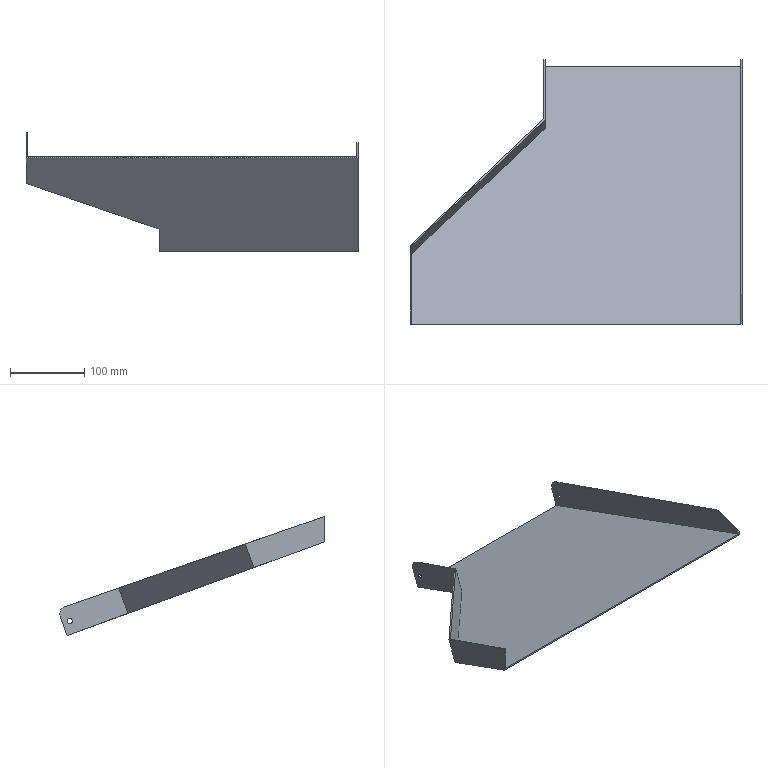Part | NX | features HB 2 | 1 solid | 19 faces | box 446 x 355.386 x 159.875 mm | volume 316995 mm3 | plane 15 | cylinder 4 | commonest cylinder face diameters 7 x2 20 x2
STEP:
#1=CARTESIAN_POINT('',(560.,345.,-264.005));
#2=VERTEX_POINT('',#1);
#3=CARTESIAN_POINT('',(118.,345.,-264.005));
#4=VERTEX_POINT('',#3);
#5=CARTESIAN_POINT('',(650.,345.,-264.005));
#6=DIRECTION('',(-1.,0.,0.));
#7=VECTOR('',#6,1000.);
#8=LINE('',#5,#7);
#9=EDGE_CURVE('',#2,#4,#8,.T.);
#10=ORIENTED_EDGE('',*,*,#9,.F.);
#11=CARTESIAN_POINT('',(560.,691.161,-389.998));
#12=VERTEX_POINT('',#11);
#13=CARTESIAN_POINT('',(560.,379.611,-276.603));
#14=DIRECTION('',(0.,0.9397,-0.342));
#15=VECTOR('',#14,1000.);
#16=LINE('',#13,#15);
#17=EDGE_CURVE('',#2,#12,#16,.T.);
#18=ORIENTED_EDGE('',*,*,#17,.T.);
#19=CARTESIAN_POINT('',(298.,691.161,-389.998));
#20=VERTEX_POINT('',#19);
#21=CARTESIAN_POINT('',(258.,691.161,-389.998));
#22=DIRECTION('',(1.,0.,0.));
#23=VECTOR('',#22,1000.);
#24=LINE('',#21,#23);
#25=EDGE_CURVE('',#20,#12,#24,.T.);
#26=ORIENTED_EDGE('',*,*,#25,.F.);
#27=CARTESIAN_POINT('',(298.,608.554,-359.931));
#28=VERTEX_POINT('',#27);
#29=CARTESIAN_POINT('',(298.,379.611,-276.603));
#30=DIRECTION('',(0.,-0.9397,0.342));
#31=VECTOR('',#30,1000.);
#32=LINE('',#29,#31);
#33=EDGE_CURVE('',#20,#28,#32,.T.);
#34=ORIENTED_EDGE('',*,*,#33,.T.);
#35=CARTESIAN_POINT('',(118.,439.409,-298.367));
#36=VERTEX_POINT('',#35);
#37=CARTESIAN_POINT('',(133.682,454.145,-303.731));
#38=DIRECTION('',(-0.7071,-0.6645,0.2418));
#39=VECTOR('',#38,1000.);
#40=LINE('',#37,#39);
#41=EDGE_CURVE('',#28,#36,#40,.T.);
#42=ORIENTED_EDGE('',*,*,#41,.T.);
#43=CARTESIAN_POINT('',(118.,379.611,-276.603));
#44=DIRECTION('',(0.,-0.9397,0.342));
#45=VECTOR('',#44,1000.);
#46=LINE('',#43,#45);
#47=EDGE_CURVE('',#36,#4,#46,.T.);
#48=ORIENTED_EDGE('',*,*,#47,.T.);
#49=EDGE_LOOP('',(#10,#18,#26,#34,#42,#48));
#50=FACE_BOUND('',#49,.T.);
#51=CARTESIAN_POINT('',(258.,379.611,-276.603));
#52=DIRECTION('',(0.,0.342,0.9397));
#53=DIRECTION('',(1.,0.,0.));
#54=AXIS2_PLACEMENT_3D('',#51,#52,#53);
#55=PLANE('',#54);
#56=ADVANCED_FACE('',(#50),#55,.T.);
#57=CARTESIAN_POINT('',(560.,345.,-260.721));
#58=VERTEX_POINT('',#57);
#59=CARTESIAN_POINT('',(560.,345.,60.));
#60=DIRECTION('',(0.,0.,-1.));
#61=VECTOR('',#60,1000.);
#62=LINE('',#59,#61);
#63=EDGE_CURVE('',#58,#2,#62,.T.);
#64=ORIENTED_EDGE('',*,*,#63,.T.);
#65=ORIENTED_EDGE('',*,*,#9,.T.);
#66=CARTESIAN_POINT('',(118.,345.,-232.002));
#67=VERTEX_POINT('',#66);
#68=CARTESIAN_POINT('',(118.,345.,60.));
#69=DIRECTION('',(0.,0.,1.));
#70=VECTOR('',#69,1000.);
#71=LINE('',#68,#70);
#72=EDGE_CURVE('',#4,#67,#71,.T.);
#73=ORIENTED_EDGE('',*,*,#72,.T.);
#74=CARTESIAN_POINT('',(116.,345.,-232.002));
#75=VERTEX_POINT('',#74);
#76=CARTESIAN_POINT('',(650.,345.,-232.002));
#77=DIRECTION('',(1.,0.,0.));
#78=VECTOR('',#77,1000.);
#79=LINE('',#76,#78);
#80=EDGE_CURVE('',#75,#67,#79,.T.);
#81=ORIENTED_EDGE('',*,*,#80,.F.);
#82=CARTESIAN_POINT('',(116.,345.,-266.134));
#83=VERTEX_POINT('',#82);
#84=CARTESIAN_POINT('',(116.,345.,60.));
#85=DIRECTION('',(0.,0.,1.));
#86=VECTOR('',#85,1000.);
#87=LINE('',#84,#86);
#88=EDGE_CURVE('',#83,#75,#87,.T.);
#89=ORIENTED_EDGE('',*,*,#88,.F.);
#90=CARTESIAN_POINT('',(562.,345.,-266.134));
#91=VERTEX_POINT('',#90);
#92=CARTESIAN_POINT('',(650.,345.,-266.134));
#93=DIRECTION('',(-1.,0.,0.));
#94=VECTOR('',#93,1000.);
#95=LINE('',#92,#94);
#96=EDGE_CURVE('',#91,#83,#95,.T.);
#97=ORIENTED_EDGE('',*,*,#96,.F.);
#98=CARTESIAN_POINT('',(562.,345.,-260.721));
#99=VERTEX_POINT('',#98);
#100=CARTESIAN_POINT('',(562.,345.,60.));
#101=DIRECTION('',(0.,0.,-1.));
#102=VECTOR('',#101,1000.);
#103=LINE('',#100,#102);
#104=EDGE_CURVE('',#99,#91,#103,.T.);
#105=ORIENTED_EDGE('',*,*,#104,.F.);
#106=CARTESIAN_POINT('',(650.,345.,-260.721));
#107=DIRECTION('',(-1.,0.,0.));
#108=VECTOR('',#107,1000.);
#109=LINE('',#106,#108);
#110=EDGE_CURVE('',#99,#58,#109,.T.);
#111=ORIENTED_EDGE('',*,*,#110,.T.);
#112=EDGE_LOOP('',(#64,#65,#73,#81,#89,#97,#105,#111));
#113=FACE_BOUND('',#112,.T.);
#114=CARTESIAN_POINT('',(650.,345.,60.));
#115=DIRECTION('',(0.,-1.,0.));
#116=DIRECTION('',(0.,0.,-1.));
#117=AXIS2_PLACEMENT_3D('',#114,#115,#116);
#118=PLANE('',#117);
#119=ADVANCED_FACE('',(#113),#118,.T.);
#120=CARTESIAN_POINT('',(562.,686.966,-375.785));
#121=VERTEX_POINT('',#120);
#122=CARTESIAN_POINT('',(562.,686.966,-372.285));
#123=DIRECTION('',(1.,0.,0.));
#124=DIRECTION('',(0.,0.,-1.));
#125=AXIS2_PLACEMENT_3D('',#122,#123,#124);
#126=CIRCLE('',#125,3.5);
#127=EDGE_CURVE('',#121,#121,#126,.T.);
#128=ORIENTED_EDGE('',*,*,#127,.F.);
#129=EDGE_LOOP('',(#128));
#130=FACE_BOUND('',#129,.T.);
#131=CARTESIAN_POINT('',(562.,385.321,-246.045));
#132=VERTEX_POINT('',#131);
#133=CARTESIAN_POINT('',(562.,370.458,-251.455));
#134=DIRECTION('',(0.,0.9397,0.342));
#135=VECTOR('',#134,1000.);
#136=LINE('',#133,#135);
#137=EDGE_CURVE('',#99,#132,#136,.T.);
#138=ORIENTED_EDGE('',*,*,#137,.F.);
#139=ORIENTED_EDGE('',*,*,#104,.T.);
#140=CARTESIAN_POINT('',(562.,690.477,-391.877));
#141=VERTEX_POINT('',#140);
#142=CARTESIAN_POINT('',(562.,378.927,-278.482));
#143=DIRECTION('',(0.,-0.9397,0.342));
#144=VECTOR('',#143,1000.);
#145=LINE('',#142,#144);
#146=EDGE_CURVE('',#141,#91,#145,.T.);
#147=ORIENTED_EDGE('',*,*,#146,.F.);
#148=CARTESIAN_POINT('',(562.,699.783,-366.309));
#149=VERTEX_POINT('',#148);
#150=CARTESIAN_POINT('',(562.,692.943,-385.102));
#151=DIRECTION('',(0.,0.342,0.9397));
#152=VECTOR('',#151,1000.);
#153=LINE('',#150,#152);
#154=EDGE_CURVE('',#141,#149,#153,.T.);
#155=ORIENTED_EDGE('',*,*,#154,.T.);
#156=CARTESIAN_POINT('',(562.,693.675,-353.445));
#157=VERTEX_POINT('',#156);
#158=CARTESIAN_POINT('',(562.,690.386,-362.888));
#159=DIRECTION('',(-1.,0.,0.));
#160=DIRECTION('',(0.,0.,1.));
#161=AXIS2_PLACEMENT_3D('',#158,#159,#160);
#162=CIRCLE('',#161,10.);
#163=EDGE_CURVE('',#157,#149,#162,.T.);
#164=ORIENTED_EDGE('',*,*,#163,.F.);
#165=CARTESIAN_POINT('',(562.,390.115,-247.715));
#166=DIRECTION('',(0.,-0.9444,0.3289));
#167=VECTOR('',#166,1000.);
#168=LINE('',#165,#167);
#169=EDGE_CURVE('',#157,#132,#168,.T.);
#170=ORIENTED_EDGE('',*,*,#169,.T.);
#171=EDGE_LOOP('',(#138,#139,#147,#155,#164,#170));
#172=FACE_BOUND('',#171,.T.);
#173=CARTESIAN_POINT('',(562.,379.611,-276.603));
#174=DIRECTION('',(-1.,0.,0.));
#175=DIRECTION('',(0.,-0.08716,0.9962));
#176=AXIS2_PLACEMENT_3D('',#173,#174,#175);
#177=PLANE('',#176);
#178=ADVANCED_FACE('',(#130,#172),#177,.F.);
#179=CARTESIAN_POINT('',(560.,385.321,-246.045));
#180=VERTEX_POINT('',#179);
#181=CARTESIAN_POINT('',(570.,385.321,-246.045));
#182=DIRECTION('',(-1.,0.,0.));
#183=VECTOR('',#182,1000.);
#184=LINE('',#181,#183);
#185=EDGE_CURVE('',#132,#180,#184,.T.);
#186=ORIENTED_EDGE('',*,*,#185,.F.);
#187=ORIENTED_EDGE('',*,*,#169,.F.);
#188=CARTESIAN_POINT('',(560.,693.675,-353.445));
#189=VERTEX_POINT('',#188);
#190=CARTESIAN_POINT('',(570.,693.675,-353.445));
#191=DIRECTION('',(1.,0.,0.));
#192=VECTOR('',#191,1000.);
#193=LINE('',#190,#192);
#194=EDGE_CURVE('',#189,#157,#193,.T.);
#195=ORIENTED_EDGE('',*,*,#194,.F.);
#196=CARTESIAN_POINT('',(560.,390.115,-247.715));
#197=DIRECTION('',(0.,-0.9444,0.3289));
#198=VECTOR('',#197,1000.);
#199=LINE('',#196,#198);
#200=EDGE_CURVE('',#189,#180,#199,.T.);
#201=ORIENTED_EDGE('',*,*,#200,.T.);
#202=EDGE_LOOP('',(#186,#187,#195,#201));
#203=FACE_BOUND('',#202,.T.);
#204=CARTESIAN_POINT('',(570.,390.115,-247.715));
#205=DIRECTION('',(0.,-0.3289,-0.9444));
#206=DIRECTION('',(0.,0.9444,-0.3289));
#207=AXIS2_PLACEMENT_3D('',#204,#205,#206);
#208=PLANE('',#207);
#209=ADVANCED_FACE('',(#203),#208,.F.);
#210=ORIENTED_EDGE('',*,*,#63,.F.);
#211=CARTESIAN_POINT('',(560.,370.458,-251.455));
#212=DIRECTION('',(0.,0.9397,0.342));
#213=VECTOR('',#212,1000.);
#214=LINE('',#211,#213);
#215=EDGE_CURVE('',#58,#180,#214,.T.);
#216=ORIENTED_EDGE('',*,*,#215,.T.);
#217=ORIENTED_EDGE('',*,*,#200,.F.);
#218=CARTESIAN_POINT('',(560.,699.783,-366.309));
#219=VERTEX_POINT('',#218);
#220=CARTESIAN_POINT('',(560.,690.386,-362.888));
#221=DIRECTION('',(1.,0.,0.));
#222=DIRECTION('',(0.,0.,1.));
#223=AXIS2_PLACEMENT_3D('',#220,#221,#222);
#224=CIRCLE('',#223,10.);
#225=EDGE_CURVE('',#219,#189,#224,.T.);
#226=ORIENTED_EDGE('',*,*,#225,.F.);
#227=CARTESIAN_POINT('',(560.,692.943,-385.102));
#228=DIRECTION('',(0.,0.342,0.9397));
#229=VECTOR('',#228,1000.);
#230=LINE('',#227,#229);
#231=EDGE_CURVE('',#12,#219,#230,.T.);
#232=ORIENTED_EDGE('',*,*,#231,.F.);
#233=ORIENTED_EDGE('',*,*,#17,.F.);
#234=EDGE_LOOP('',(#210,#216,#217,#226,#232,#233));
#235=FACE_BOUND('',#234,.T.);
#236=CARTESIAN_POINT('',(560.,686.966,-375.785));
#237=VERTEX_POINT('',#236);
#238=CARTESIAN_POINT('',(560.,686.966,-372.285));
#239=DIRECTION('',(-1.,0.,0.));
#240=DIRECTION('',(0.,0.,-1.));
#241=AXIS2_PLACEMENT_3D('',#238,#239,#240);
#242=CIRCLE('',#241,3.5);
#243=EDGE_CURVE('',#237,#237,#242,.T.);
#244=ORIENTED_EDGE('',*,*,#243,.F.);
#245=EDGE_LOOP('',(#244));
#246=FACE_BOUND('',#245,.T.);
#247=CARTESIAN_POINT('',(560.,379.611,-276.603));
#248=DIRECTION('',(-1.,0.,0.));
#249=DIRECTION('',(0.,-0.08716,0.9962));
#250=AXIS2_PLACEMENT_3D('',#247,#248,#249);
#251=PLANE('',#250);
#252=ADVANCED_FACE('',(#235,#246),#251,.T.);
#253=CARTESIAN_POINT('',(118.,450.225,-268.651));
#254=VERTEX_POINT('',#253);
#255=CARTESIAN_POINT('',(118.,449.669,-270.177));
#256=DIRECTION('',(0.,0.342,0.9397));
#257=VECTOR('',#256,1000.);
#258=LINE('',#255,#257);
#259=EDGE_CURVE('',#36,#254,#258,.T.);
#260=ORIENTED_EDGE('',*,*,#259,.T.);
#261=CARTESIAN_POINT('',(118.,390.115,-247.715));
#262=DIRECTION('',(0.,-0.9444,0.3289));
#263=VECTOR('',#262,1000.);
#264=LINE('',#261,#263);
#265=EDGE_CURVE('',#254,#67,#264,.T.);
#266=ORIENTED_EDGE('',*,*,#265,.T.);
#267=ORIENTED_EDGE('',*,*,#72,.F.);
#268=ORIENTED_EDGE('',*,*,#47,.F.);
#269=EDGE_LOOP('',(#260,#266,#267,#268));
#270=FACE_BOUND('',#269,.T.);
#271=CARTESIAN_POINT('',(118.,379.611,-276.603));
#272=DIRECTION('',(1.,0.,0.));
#273=DIRECTION('',(0.,-0.08716,0.9962));
#274=AXIS2_PLACEMENT_3D('',#271,#272,#273);
#275=PLANE('',#274);
#276=ADVANCED_FACE('',(#270),#275,.T.);
#277=CARTESIAN_POINT('',(296.,608.648,-362.094));
#278=VERTEX_POINT('',#277);
#279=CARTESIAN_POINT('',(116.,439.503,-300.53));
#280=VERTEX_POINT('',#279);
#281=CARTESIAN_POINT('',(132.268,454.79,-306.094));
#282=DIRECTION('',(-0.7071,-0.6645,0.2418));
#283=VECTOR('',#282,1000.);
#284=LINE('',#281,#283);
#285=EDGE_CURVE('',#278,#280,#284,.T.);
#286=ORIENTED_EDGE('',*,*,#285,.F.);
#287=CARTESIAN_POINT('',(296.,690.477,-391.877));
#288=VERTEX_POINT('',#287);
#289=CARTESIAN_POINT('',(296.,378.927,-278.482));
#290=DIRECTION('',(0.,0.9397,-0.342));
#291=VECTOR('',#290,1000.);
#292=LINE('',#289,#291);
#293=EDGE_CURVE('',#278,#288,#292,.T.);
#294=ORIENTED_EDGE('',*,*,#293,.T.);
#295=CARTESIAN_POINT('',(258.,690.477,-391.877));
#296=DIRECTION('',(1.,0.,0.));
#297=VECTOR('',#296,1000.);
#298=LINE('',#295,#297);
#299=EDGE_CURVE('',#288,#141,#298,.T.);
#300=ORIENTED_EDGE('',*,*,#299,.T.);
#301=ORIENTED_EDGE('',*,*,#146,.T.);
#302=ORIENTED_EDGE('',*,*,#96,.T.);
#303=CARTESIAN_POINT('',(116.,378.927,-278.482));
#304=DIRECTION('',(0.,0.9397,-0.342));
#305=VECTOR('',#304,1000.);
#306=LINE('',#303,#305);
#307=EDGE_CURVE('',#83,#280,#306,.T.);
#308=ORIENTED_EDGE('',*,*,#307,.T.);
#309=EDGE_LOOP('',(#286,#294,#300,#301,#302,#308));
#310=FACE_BOUND('',#309,.T.);
#311=CARTESIAN_POINT('',(258.,378.927,-278.482));
#312=DIRECTION('',(0.,0.342,0.9397));
#313=DIRECTION('',(1.,0.,0.));
#314=AXIS2_PLACEMENT_3D('',#311,#312,#313);
#315=PLANE('',#314);
#316=ADVANCED_FACE('',(#310),#315,.F.);
#317=CARTESIAN_POINT('',(116.,451.007,-268.924));
#318=VERTEX_POINT('',#317);
#319=CARTESIAN_POINT('',(116.,440.187,-298.651));
#320=DIRECTION('',(0.,-0.342,-0.9397));
#321=VECTOR('',#320,1000.);
#322=LINE('',#319,#321);
#323=EDGE_CURVE('',#318,#280,#322,.T.);
#324=ORIENTED_EDGE('',*,*,#323,.T.);
#325=ORIENTED_EDGE('',*,*,#307,.F.);
#326=ORIENTED_EDGE('',*,*,#88,.T.);
#327=CARTESIAN_POINT('',(116.,390.115,-247.715));
#328=DIRECTION('',(0.,-0.9444,0.3289));
#329=VECTOR('',#328,1000.);
#330=LINE('',#327,#329);
#331=EDGE_CURVE('',#318,#75,#330,.T.);
#332=ORIENTED_EDGE('',*,*,#331,.F.);
#333=EDGE_LOOP('',(#324,#325,#326,#332));
#334=FACE_BOUND('',#333,.T.);
#335=CARTESIAN_POINT('',(116.,379.611,-276.603));
#336=DIRECTION('',(1.,0.,0.));
#337=DIRECTION('',(0.,0.08716,-0.9962));
#338=AXIS2_PLACEMENT_3D('',#335,#336,#337);
#339=PLANE('',#338);
#340=ADVANCED_FACE('',(#334),#339,.F.);
#341=CARTESIAN_POINT('',(296.,621.008,-328.135));
#342=VERTEX_POINT('',#341);
#343=CARTESIAN_POINT('',(170.983,502.936,-287.011));
#344=DIRECTION('',(0.7071,0.6678,-0.2326));
#345=VECTOR('',#344,1000.);
#346=LINE('',#343,#345);
#347=EDGE_CURVE('',#318,#342,#346,.T.);
#348=ORIENTED_EDGE('',*,*,#347,.F.);
#349=ORIENTED_EDGE('',*,*,#331,.T.);
#350=ORIENTED_EDGE('',*,*,#80,.T.);
#351=ORIENTED_EDGE('',*,*,#265,.F.);
#352=CARTESIAN_POINT('',(298.,620.226,-327.862));
#353=VERTEX_POINT('',#352);
#354=CARTESIAN_POINT('',(172.398,501.601,-286.545));
#355=DIRECTION('',(0.7071,0.6678,-0.2326));
#356=VECTOR('',#355,1000.);
#357=LINE('',#354,#356);
#358=EDGE_CURVE('',#254,#353,#357,.T.);
#359=ORIENTED_EDGE('',*,*,#358,.T.);
#360=CARTESIAN_POINT('',(298.,693.675,-353.445));
#361=VERTEX_POINT('',#360);
#362=CARTESIAN_POINT('',(298.,390.115,-247.715));
#363=DIRECTION('',(0.,-0.9444,0.3289));
#364=VECTOR('',#363,1000.);
#365=LINE('',#362,#364);
#366=EDGE_CURVE('',#361,#353,#365,.T.);
#367=ORIENTED_EDGE('',*,*,#366,.F.);
#368=CARTESIAN_POINT('',(296.,693.675,-353.445));
#369=VERTEX_POINT('',#368);
#370=CARTESIAN_POINT('',(258.,693.675,-353.445));
#371=DIRECTION('',(1.,0.,0.));
#372=VECTOR('',#371,1000.);
#373=LINE('',#370,#372);
#374=EDGE_CURVE('',#369,#361,#373,.T.);
#375=ORIENTED_EDGE('',*,*,#374,.F.);
#376=CARTESIAN_POINT('',(296.,390.115,-247.715));
#377=DIRECTION('',(0.,-0.9444,0.3289));
#378=VECTOR('',#377,1000.);
#379=LINE('',#376,#378);
#380=EDGE_CURVE('',#369,#342,#379,.T.);
#381=ORIENTED_EDGE('',*,*,#380,.T.);
#382=EDGE_LOOP('',(#348,#349,#350,#351,#359,#367,#375,#381));
#383=FACE_BOUND('',#382,.T.);
#384=CARTESIAN_POINT('',(218.,390.115,-247.715));
#385=DIRECTION('',(0.,-0.3289,-0.9444));
#386=DIRECTION('',(0.,0.9444,-0.3289));
#387=AXIS2_PLACEMENT_3D('',#384,#385,#386);
#388=PLANE('',#387);
#389=ADVANCED_FACE('',(#383),#388,.F.);
#390=ORIENTED_EDGE('',*,*,#366,.T.);
#391=CARTESIAN_POINT('',(298.,608.554,-359.931));
#392=DIRECTION('',(0.,-0.342,-0.9397));
#393=VECTOR('',#392,1000.);
#394=LINE('',#391,#393);
#395=EDGE_CURVE('',#353,#28,#394,.T.);
#396=ORIENTED_EDGE('',*,*,#395,.T.);
#397=ORIENTED_EDGE('',*,*,#33,.F.);
#398=CARTESIAN_POINT('',(298.,699.783,-366.309));
#399=VERTEX_POINT('',#398);
#400=CARTESIAN_POINT('',(298.,692.943,-385.102));
#401=DIRECTION('',(0.,0.342,0.9397));
#402=VECTOR('',#401,1000.);
#403=LINE('',#400,#402);
#404=EDGE_CURVE('',#20,#399,#403,.T.);
#405=ORIENTED_EDGE('',*,*,#404,.T.);
#406=CARTESIAN_POINT('',(298.,690.386,-362.888));
#407=DIRECTION('',(-1.,0.,0.));
#408=DIRECTION('',(0.,0.,-1.));
#409=AXIS2_PLACEMENT_3D('',#406,#407,#408);
#410=CIRCLE('',#409,10.);
#411=EDGE_CURVE('',#361,#399,#410,.T.);
#412=ORIENTED_EDGE('',*,*,#411,.F.);
#413=EDGE_LOOP('',(#390,#396,#397,#405,#412));
#414=FACE_BOUND('',#413,.T.);
#415=CARTESIAN_POINT('',(298.,686.661,-368.799));
#416=VERTEX_POINT('',#415);
#417=CARTESIAN_POINT('',(298.,686.966,-372.285));
#418=DIRECTION('',(1.,0.,0.));
#419=DIRECTION('',(0.,-0.08716,0.9962));
#420=AXIS2_PLACEMENT_3D('',#417,#418,#419);
#421=CIRCLE('',#420,3.5);
#422=EDGE_CURVE('',#416,#416,#421,.T.);
#423=ORIENTED_EDGE('',*,*,#422,.F.);
#424=EDGE_LOOP('',(#423));
#425=FACE_BOUND('',#424,.T.);
#426=CARTESIAN_POINT('',(298.,379.611,-276.603));
#427=DIRECTION('',(1.,0.,0.));
#428=DIRECTION('',(0.,-0.08716,0.9962));
#429=AXIS2_PLACEMENT_3D('',#426,#427,#428);
#430=PLANE('',#429);
#431=ADVANCED_FACE('',(#414,#425),#430,.T.);
#432=CARTESIAN_POINT('',(296.,686.661,-368.799));
#433=VERTEX_POINT('',#432);
#434=CARTESIAN_POINT('',(296.,686.966,-372.285));
#435=DIRECTION('',(1.,0.,0.));
#436=DIRECTION('',(0.,-0.08716,0.9962));
#437=AXIS2_PLACEMENT_3D('',#434,#435,#436);
#438=CIRCLE('',#437,3.5);
#439=EDGE_CURVE('',#433,#433,#438,.T.);
#440=ORIENTED_EDGE('',*,*,#439,.T.);
#441=EDGE_LOOP('',(#440));
#442=FACE_BOUND('',#441,.T.);
#443=ORIENTED_EDGE('',*,*,#293,.F.);
#444=CARTESIAN_POINT('',(296.,609.332,-360.214));
#445=DIRECTION('',(0.,-0.342,-0.9397));
#446=VECTOR('',#445,1000.);
#447=LINE('',#444,#446);
#448=EDGE_CURVE('',#342,#278,#447,.T.);
#449=ORIENTED_EDGE('',*,*,#448,.F.);
#450=ORIENTED_EDGE('',*,*,#380,.F.);
#451=CARTESIAN_POINT('',(296.,699.783,-366.309));
#452=VERTEX_POINT('',#451);
#453=CARTESIAN_POINT('',(296.,690.386,-362.888));
#454=DIRECTION('',(1.,0.,0.));
#455=DIRECTION('',(0.,0.,-1.));
#456=AXIS2_PLACEMENT_3D('',#453,#454,#455);
#457=CIRCLE('',#456,10.);
#458=EDGE_CURVE('',#452,#369,#457,.T.);
#459=ORIENTED_EDGE('',*,*,#458,.F.);
#460=CARTESIAN_POINT('',(296.,692.943,-385.102));
#461=DIRECTION('',(0.,0.342,0.9397));
#462=VECTOR('',#461,1000.);
#463=LINE('',#460,#462);
#464=EDGE_CURVE('',#288,#452,#463,.T.);
#465=ORIENTED_EDGE('',*,*,#464,.F.);
#466=EDGE_LOOP('',(#443,#449,#450,#459,#465));
#467=FACE_BOUND('',#466,.T.);
#468=CARTESIAN_POINT('',(296.,379.611,-276.603));
#469=DIRECTION('',(1.,0.,0.));
#470=DIRECTION('',(0.,0.08716,-0.9962));
#471=AXIS2_PLACEMENT_3D('',#468,#469,#470);
#472=PLANE('',#471);
#473=ADVANCED_FACE('',(#442,#467),#472,.F.);
#474=ORIENTED_EDGE('',*,*,#422,.T.);
#475=EDGE_LOOP('',(#474));
#476=FACE_BOUND('',#475,.T.);
#477=ORIENTED_EDGE('',*,*,#439,.F.);
#478=EDGE_LOOP('',(#477));
#479=FACE_BOUND('',#478,.T.);
#480=CARTESIAN_POINT('',(-406.,686.966,-372.285));
#481=DIRECTION('',(1.,0.,0.));
#482=DIRECTION('',(0.,0.08716,-0.9962));
#483=AXIS2_PLACEMENT_3D('',#480,#481,#482);
#484=CYLINDRICAL_SURFACE('',#483,3.5);
#485=ADVANCED_FACE('',(#476,#479),#484,.F.);
#486=ORIENTED_EDGE('',*,*,#411,.T.);
#487=CARTESIAN_POINT('',(258.,699.783,-366.309));
#488=DIRECTION('',(-1.,0.,0.));
#489=VECTOR('',#488,1000.);
#490=LINE('',#487,#489);
#491=EDGE_CURVE('',#399,#452,#490,.T.);
#492=ORIENTED_EDGE('',*,*,#491,.T.);
#493=ORIENTED_EDGE('',*,*,#458,.T.);
#494=ORIENTED_EDGE('',*,*,#374,.T.);
#495=EDGE_LOOP('',(#486,#492,#493,#494));
#496=FACE_BOUND('',#495,.T.);
#497=CARTESIAN_POINT('',(258.,690.386,-362.888));
#498=DIRECTION('',(1.,0.,0.));
#499=DIRECTION('',(0.,0.,1.));
#500=AXIS2_PLACEMENT_3D('',#497,#498,#499);
#501=CYLINDRICAL_SURFACE('',#500,10.);
#502=ADVANCED_FACE('',(#496),#501,.T.);
#503=ORIENTED_EDGE('',*,*,#25,.T.);
#504=ORIENTED_EDGE('',*,*,#231,.T.);
#505=CARTESIAN_POINT('',(570.,699.783,-366.309));
#506=DIRECTION('',(-1.,0.,0.));
#507=VECTOR('',#506,1000.);
#508=LINE('',#505,#507);
#509=EDGE_CURVE('',#149,#219,#508,.T.);
#510=ORIENTED_EDGE('',*,*,#509,.F.);
#511=ORIENTED_EDGE('',*,*,#154,.F.);
#512=ORIENTED_EDGE('',*,*,#299,.F.);
#513=ORIENTED_EDGE('',*,*,#464,.T.);
#514=ORIENTED_EDGE('',*,*,#491,.F.);
#515=ORIENTED_EDGE('',*,*,#404,.F.);
#516=EDGE_LOOP('',(#503,#504,#510,#511,#512,#513,#514,#515));
#517=FACE_BOUND('',#516,.T.);
#518=CARTESIAN_POINT('',(258.,692.943,-385.102));
#519=DIRECTION('',(0.,-0.9397,0.342));
#520=DIRECTION('',(0.,-0.342,-0.9397));
#521=AXIS2_PLACEMENT_3D('',#518,#519,#520);
#522=PLANE('',#521);
#523=ADVANCED_FACE('',(#517),#522,.F.);
#524=ORIENTED_EDGE('',*,*,#225,.T.);
#525=ORIENTED_EDGE('',*,*,#194,.T.);
#526=ORIENTED_EDGE('',*,*,#163,.T.);
#527=ORIENTED_EDGE('',*,*,#509,.T.);
#528=EDGE_LOOP('',(#524,#525,#526,#527));
#529=FACE_BOUND('',#528,.T.);
#530=CARTESIAN_POINT('',(570.,690.386,-362.888));
#531=DIRECTION('',(-1.,0.,0.));
#532=DIRECTION('',(0.,0.,-1.));
#533=AXIS2_PLACEMENT_3D('',#530,#531,#532);
#534=CYLINDRICAL_SURFACE('',#533,10.);
#535=ADVANCED_FACE('',(#529),#534,.T.);
#536=ORIENTED_EDGE('',*,*,#243,.T.);
#537=EDGE_LOOP('',(#536));
#538=FACE_BOUND('',#537,.T.);
#539=ORIENTED_EDGE('',*,*,#127,.T.);
#540=EDGE_LOOP('',(#539));
#541=FACE_BOUND('',#540,.T.);
#542=CARTESIAN_POINT('',(-335.,686.966,-372.285));
#543=DIRECTION('',(1.,0.,0.));
#544=DIRECTION('',(0.,0.08716,-0.9962));
#545=AXIS2_PLACEMENT_3D('',#542,#543,#544);
#546=CYLINDRICAL_SURFACE('',#545,3.5);
#547=ADVANCED_FACE('',(#538,#541),#546,.F.);
#548=ORIENTED_EDGE('',*,*,#448,.T.);
#549=ORIENTED_EDGE('',*,*,#285,.T.);
#550=ORIENTED_EDGE('',*,*,#323,.F.);
#551=ORIENTED_EDGE('',*,*,#347,.T.);
#552=EDGE_LOOP('',(#548,#549,#550,#551));
#553=FACE_BOUND('',#552,.T.);
#554=CARTESIAN_POINT('',(171.,502.131,-289.271));
#555=DIRECTION('',(0.7071,-0.6645,0.2418));
#556=DIRECTION('',(0.,0.342,0.9397));
#557=AXIS2_PLACEMENT_3D('',#554,#555,#556);
#558=PLANE('',#557);
#559=ADVANCED_FACE('',(#553),#558,.F.);
#560=ORIENTED_EDGE('',*,*,#259,.F.);
#561=ORIENTED_EDGE('',*,*,#41,.F.);
#562=ORIENTED_EDGE('',*,*,#395,.F.);
#563=ORIENTED_EDGE('',*,*,#358,.F.);
#564=EDGE_LOOP('',(#560,#561,#562,#563));
#565=FACE_BOUND('',#564,.T.);
#566=CARTESIAN_POINT('',(172.414,500.802,-288.787));
#567=DIRECTION('',(0.7071,-0.6645,0.2418));
#568=DIRECTION('',(0.,0.342,0.9397));
#569=AXIS2_PLACEMENT_3D('',#566,#567,#568);
#570=PLANE('',#569);
#571=ADVANCED_FACE('',(#565),#570,.T.);
#572=ORIENTED_EDGE('',*,*,#215,.F.);
#573=ORIENTED_EDGE('',*,*,#110,.F.);
#574=ORIENTED_EDGE('',*,*,#137,.T.);
#575=ORIENTED_EDGE('',*,*,#185,.T.);
#576=EDGE_LOOP('',(#572,#573,#574,#575));
#577=FACE_BOUND('',#576,.T.);
#578=CARTESIAN_POINT('',(608.54,21.454,-378.482));
#579=DIRECTION('',(0.,-0.342,0.9397));
#580=DIRECTION('',(-1.,0.,0.));
#581=AXIS2_PLACEMENT_3D('',#578,#579,#580);
#582=PLANE('',#581);
#583=ADVANCED_FACE('',(#577),#582,.T.);
#584=CLOSED_SHELL('',(#56,#119,#178,#209,#252,#276,#316,#340,#389,#431,#473,#485,#502,#523,#535,#547,#559,#571,#583));
#585=MANIFOLD_SOLID_BREP('',#584);
#586=(LENGTH_UNIT()NAMED_UNIT(*)SI_UNIT(.MILLI.,.METRE.));
#587=UNCERTAINTY_MEASURE_WITH_UNIT(LENGTH_MEASURE(0.00001),#586,'','');
#588=(NAMED_UNIT(*)PLANE_ANGLE_UNIT()SI_UNIT($,.RADIAN.));
#589=(NAMED_UNIT(*)SI_UNIT($,.STERADIAN.)SOLID_ANGLE_UNIT());
#590=(GEOMETRIC_REPRESENTATION_CONTEXT(3)GLOBAL_UNCERTAINTY_ASSIGNED_CONTEXT((#587))GLOBAL_UNIT_ASSIGNED_CONTEXT((#586,#588,#589))REPRESENTATION_CONTEXT('',''));
#591=ADVANCED_BREP_SHAPE_REPRESENTATION('',(#585),#590);